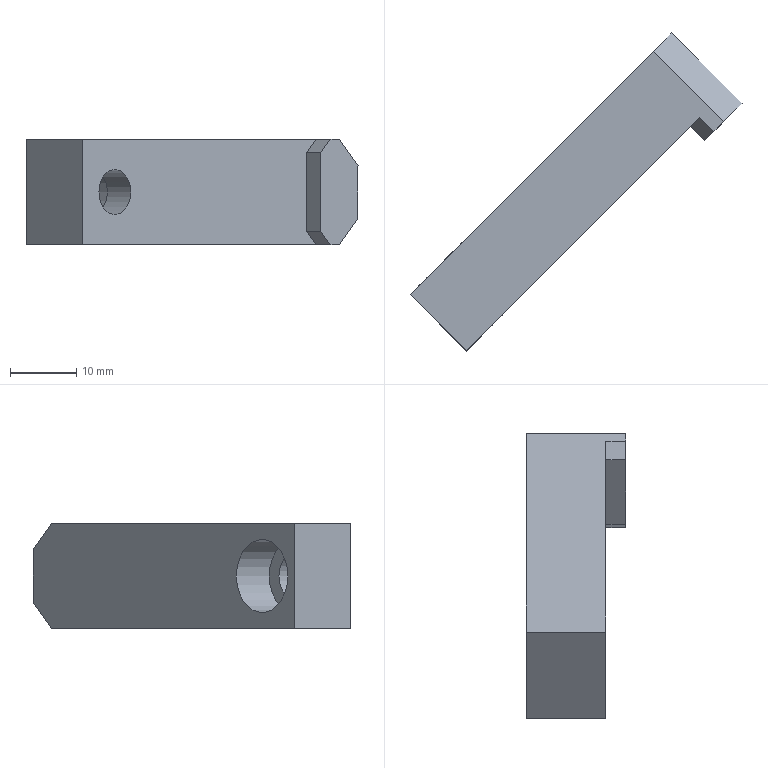Part | STEP file | gslz 2016.10.28-13_id1394_x_t | 1 solid | 15 faces | box 50.205 x 48.083 x 16 mm | volume 10037 mm3 | plane 13 | cylinder 2 | commonest cylinder face diameters 6.8 x1 11 x1
STEP:
#1=CARTESIAN_POINT('',(0.,0.,0.));
#2=DIRECTION('',(0.,0.,1.));
#3=DIRECTION('',(1.,0.,0.));
#4=AXIS2_PLACEMENT_3D('',#1,#2,#3);
#5=CARTESIAN_POINT('',(579.881,214.556,-16.623));
#6=VERTEX_POINT('',#5);
#7=CARTESIAN_POINT('',(578.467,213.142,-16.623));
#8=VERTEX_POINT('',#7);
#9=CARTESIAN_POINT('',(582.003,216.678,-16.623));
#10=DIRECTION('',(-0.7071,-0.7071,0.));
#11=VECTOR('',#10,1.);
#12=LINE('',#9,#11);
#13=CARTESIAN_POINT('',(562.204,215.264,-16.623));
#14=DIRECTION('',(0.,0.,-1.));
#15=DIRECTION('',(-0.766,0.6428,0.));
#16=AXIS2_PLACEMENT_3D('',#13,#14,#15);
#17=PLANE('',#16);
#18=CARTESIAN_POINT('',(-14.258,13.81));
#19=DIRECTION('',(0.08716,-0.9962));
#20=VECTOR('',#19,1.);
#21=LINE('',#18,#20);
#22=(GEOMETRIC_REPRESENTATION_CONTEXT(2)PARAMETRIC_REPRESENTATION_CONTEXT()REPRESENTATION_CONTEXT('',''));
#23=DEFINITIONAL_REPRESENTATION('',(#21),#22);
#24=PCURVE('',#17,#23);
#25=CARTESIAN_POINT('',(578.467,213.142,-46.123));
#26=DIRECTION('',(-0.7071,0.7071,0.));
#27=DIRECTION('',(-0.7071,-0.7071,0.));
#28=AXIS2_PLACEMENT_3D('',#25,#26,#27);
#29=PLANE('',#28);
#30=CARTESIAN_POINT('',(-5.,29.5));
#31=DIRECTION('',(1.,0.));
#32=VECTOR('',#31,1.);
#33=LINE('',#30,#32);
#34=(GEOMETRIC_REPRESENTATION_CONTEXT(2)PARAMETRIC_REPRESENTATION_CONTEXT()REPRESENTATION_CONTEXT('',''));
#35=DEFINITIONAL_REPRESENTATION('',(#33),#34);
#36=PCURVE('',#29,#35);
#37=SURFACE_CURVE('',#12,(#24,#36),.PCURVE_S1.);
#38=EDGE_CURVE('',#6,#8,#37,.T.);
#39=ORIENTED_EDGE('',*,*,#38,.F.);
#40=CARTESIAN_POINT('',(569.275,225.163,-16.623));
#41=VERTEX_POINT('',#40);
#42=CARTESIAN_POINT('',(569.275,225.163,-16.623));
#43=DIRECTION('',(-0.7071,0.7071,0.));
#44=VECTOR('',#43,1.);
#45=LINE('',#42,#44);
#46=CARTESIAN_POINT('',(0.9465,12.129));
#47=DIRECTION('',(0.9962,0.08716));
#48=VECTOR('',#47,1.);
#49=LINE('',#46,#48);
#50=(GEOMETRIC_REPRESENTATION_CONTEXT(2)PARAMETRIC_REPRESENTATION_CONTEXT()REPRESENTATION_CONTEXT('',''));
#51=DEFINITIONAL_REPRESENTATION('',(#49),#50);
#52=PCURVE('',#17,#51);
#53=CARTESIAN_POINT('',(570.689,223.749,-16.623));
#54=DIRECTION('',(0.5,0.5,0.7071));
#55=DIRECTION('',(0.7071,-0.7071,0.));
#56=AXIS2_PLACEMENT_3D('',#53,#54,#55);
#57=PLANE('',#56);
#58=CARTESIAN_POINT('',(-2.,0.));
#59=DIRECTION('',(-1.,0.));
#60=VECTOR('',#59,1.);
#61=LINE('',#58,#60);
#62=(GEOMETRIC_REPRESENTATION_CONTEXT(2)PARAMETRIC_REPRESENTATION_CONTEXT()REPRESENTATION_CONTEXT('',''));
#63=DEFINITIONAL_REPRESENTATION('',(#61),#62);
#64=PCURVE('',#57,#63);
#65=SURFACE_CURVE('',#45,(#52,#64),.PCURVE_S1.);
#66=EDGE_CURVE('',#6,#41,#65,.T.);
#67=ORIENTED_EDGE('',*,*,#66,.T.);
#68=CARTESIAN_POINT('',(532.505,188.393,-16.623));
#69=VERTEX_POINT('',#68);
#70=CARTESIAN_POINT('',(560.789,216.678,-16.623));
#71=DIRECTION('',(-0.7071,-0.7071,0.));
#72=VECTOR('',#71,1.);
#73=LINE('',#70,#72);
#74=CARTESIAN_POINT('',(1.992,0.1743));
#75=DIRECTION('',(0.08716,-0.9962));
#76=VECTOR('',#75,1.);
#77=LINE('',#74,#76);
#78=(GEOMETRIC_REPRESENTATION_CONTEXT(2)PARAMETRIC_REPRESENTATION_CONTEXT()REPRESENTATION_CONTEXT('',''));
#79=DEFINITIONAL_REPRESENTATION('',(#77),#78);
#80=PCURVE('',#17,#79);
#81=CARTESIAN_POINT('',(560.789,216.678,-46.123));
#82=DIRECTION('',(-0.7071,0.7071,0.));
#83=DIRECTION('',(-0.7071,-0.7071,0.));
#84=AXIS2_PLACEMENT_3D('',#81,#82,#83);
#85=PLANE('',#84);
#86=CARTESIAN_POINT('',(0.,29.5));
#87=DIRECTION('',(1.,0.));
#88=VECTOR('',#87,1.);
#89=LINE('',#86,#88);
#90=(GEOMETRIC_REPRESENTATION_CONTEXT(2)PARAMETRIC_REPRESENTATION_CONTEXT()REPRESENTATION_CONTEXT('',''));
#91=DEFINITIONAL_REPRESENTATION('',(#89),#90);
#92=PCURVE('',#85,#91);
#93=SURFACE_CURVE('',#73,(#80,#92),.PCURVE_S1.);
#94=EDGE_CURVE('',#41,#69,#93,.T.);
#95=ORIENTED_EDGE('',*,*,#94,.T.);
#96=CARTESIAN_POINT('',(540.99,179.908,-16.623));
#97=VERTEX_POINT('',#96);
#98=CARTESIAN_POINT('',(533.919,186.979,-16.623));
#99=DIRECTION('',(-0.7071,0.7071,0.));
#100=VECTOR('',#99,1.);
#101=LINE('',#98,#100);
#102=CARTESIAN_POINT('',(3.486,-39.848));
#103=DIRECTION('',(0.9962,0.08716));
#104=VECTOR('',#103,1.);
#105=LINE('',#102,#104);
#106=(GEOMETRIC_REPRESENTATION_CONTEXT(2)PARAMETRIC_REPRESENTATION_CONTEXT()REPRESENTATION_CONTEXT('',''));
#107=DEFINITIONAL_REPRESENTATION('',(#105),#106);
#108=PCURVE('',#17,#107);
#109=CARTESIAN_POINT('',(533.919,186.979,-46.123));
#110=DIRECTION('',(-0.7071,-0.7071,0.));
#111=DIRECTION('',(-0.7071,0.7071,0.));
#112=AXIS2_PLACEMENT_3D('',#109,#110,#111);
#113=PLANE('',#112);
#114=CARTESIAN_POINT('',(0.,-29.5));
#115=DIRECTION('',(1.,0.));
#116=VECTOR('',#115,1.);
#117=LINE('',#114,#116);
#118=(GEOMETRIC_REPRESENTATION_CONTEXT(2)PARAMETRIC_REPRESENTATION_CONTEXT()REPRESENTATION_CONTEXT('',''));
#119=DEFINITIONAL_REPRESENTATION('',(#117),#118);
#120=PCURVE('',#113,#119);
#121=SURFACE_CURVE('',#101,(#108,#120),.PCURVE_S1.);
#122=EDGE_CURVE('',#97,#69,#121,.T.);
#123=ORIENTED_EDGE('',*,*,#122,.F.);
#124=CARTESIAN_POINT('',(576.346,215.264,-16.623));
#125=VERTEX_POINT('',#124);
#126=CARTESIAN_POINT('',(569.275,208.192,-16.623));
#127=DIRECTION('',(-0.7071,-0.7071,0.));
#128=VECTOR('',#127,1.);
#129=LINE('',#126,#128);
#130=CARTESIAN_POINT('',(-9.962,-0.8716));
#131=DIRECTION('',(0.08716,-0.9962));
#132=VECTOR('',#131,1.);
#133=LINE('',#130,#132);
#134=(GEOMETRIC_REPRESENTATION_CONTEXT(2)PARAMETRIC_REPRESENTATION_CONTEXT()REPRESENTATION_CONTEXT('',''));
#135=DEFINITIONAL_REPRESENTATION('',(#133),#134);
#136=PCURVE('',#17,#135);
#137=CARTESIAN_POINT('',(569.275,208.192,-46.123));
#138=DIRECTION('',(-0.7071,0.7071,0.));
#139=DIRECTION('',(-0.7071,-0.7071,0.));
#140=AXIS2_PLACEMENT_3D('',#137,#138,#139);
#141=PLANE('',#140);
#142=CARTESIAN_POINT('',(0.,29.5));
#143=DIRECTION('',(1.,0.));
#144=VECTOR('',#143,1.);
#145=LINE('',#142,#144);
#146=(GEOMETRIC_REPRESENTATION_CONTEXT(2)PARAMETRIC_REPRESENTATION_CONTEXT()REPRESENTATION_CONTEXT('',''));
#147=DEFINITIONAL_REPRESENTATION('',(#145),#146);
#148=PCURVE('',#141,#147);
#149=SURFACE_CURVE('',#129,(#136,#148),.PCURVE_S1.);
#150=EDGE_CURVE('',#125,#97,#149,.T.);
#151=ORIENTED_EDGE('',*,*,#150,.F.);
#152=CARTESIAN_POINT('',(569.275,222.335,-16.623));
#153=DIRECTION('',(-0.7071,0.7071,0.));
#154=VECTOR('',#153,1.);
#155=LINE('',#152,#154);
#156=CARTESIAN_POINT('',(-0.8716,9.962));
#157=DIRECTION('',(0.9962,0.08716));
#158=VECTOR('',#157,1.);
#159=LINE('',#156,#158);
#160=(GEOMETRIC_REPRESENTATION_CONTEXT(2)PARAMETRIC_REPRESENTATION_CONTEXT()REPRESENTATION_CONTEXT('',''));
#161=DEFINITIONAL_REPRESENTATION('',(#159),#160);
#162=PCURVE('',#17,#161);
#163=CARTESIAN_POINT('',(570.689,223.749,-14.623));
#164=DIRECTION('',(0.5,0.5,-0.7071));
#165=DIRECTION('',(0.7071,-0.7071,0.));
#166=AXIS2_PLACEMENT_3D('',#163,#164,#165);
#167=PLANE('',#166);
#168=CARTESIAN_POINT('',(0.,2.828));
#169=DIRECTION('',(-1.,0.));
#170=VECTOR('',#169,1.);
#171=LINE('',#168,#170);
#172=(GEOMETRIC_REPRESENTATION_CONTEXT(2)PARAMETRIC_REPRESENTATION_CONTEXT()REPRESENTATION_CONTEXT('',''));
#173=DEFINITIONAL_REPRESENTATION('',(#171),#172);
#174=PCURVE('',#167,#173);
#175=SURFACE_CURVE('',#155,(#162,#174),.PCURVE_S1.);
#176=EDGE_CURVE('',#8,#125,#175,.T.);
#177=ORIENTED_EDGE('',*,*,#176,.F.);
#178=EDGE_LOOP('',(#39,#67,#95,#123,#151,#177));
#179=FACE_BOUND('',#178,.T.);
#180=ADVANCED_FACE('',(#179),#17,.F.);
#181=CARTESIAN_POINT('',(582.71,217.385,-20.623));
#182=VERTEX_POINT('',#181);
#183=CARTESIAN_POINT('',(582.71,217.385,-28.623));
#184=VERTEX_POINT('',#183);
#185=CARTESIAN_POINT('',(582.71,217.385,-46.123));
#186=DIRECTION('',(0.,0.,-1.));
#187=VECTOR('',#186,1.);
#188=LINE('',#185,#187);
#189=CARTESIAN_POINT('',(573.517,226.577,-46.123));
#190=DIRECTION('',(0.7071,0.7071,0.));
#191=DIRECTION('',(-0.7071,0.7071,0.));
#192=AXIS2_PLACEMENT_3D('',#189,#190,#191);
#193=PLANE('',#192);
#194=CARTESIAN_POINT('',(-13.,0.));
#195=DIRECTION('',(0.,-1.));
#196=VECTOR('',#195,1.);
#197=LINE('',#194,#196);
#198=(GEOMETRIC_REPRESENTATION_CONTEXT(2)PARAMETRIC_REPRESENTATION_CONTEXT()REPRESENTATION_CONTEXT('',''));
#199=DEFINITIONAL_REPRESENTATION('',(#197),#198);
#200=PCURVE('',#193,#199);
#201=CARTESIAN_POINT('',(-6.,0.));
#202=DIRECTION('',(0.,-1.));
#203=VECTOR('',#202,1.);
#204=LINE('',#201,#203);
#205=(GEOMETRIC_REPRESENTATION_CONTEXT(2)PARAMETRIC_REPRESENTATION_CONTEXT()REPRESENTATION_CONTEXT('',''));
#206=DEFINITIONAL_REPRESENTATION('',(#204),#205);
#207=PCURVE('',#29,#206);
#208=SURFACE_CURVE('',#188,(#200,#207),.PCURVE_S1.);
#209=EDGE_CURVE('',#182,#184,#208,.T.);
#210=ORIENTED_EDGE('',*,*,#209,.T.);
#211=CARTESIAN_POINT('',(572.103,227.991,-28.623));
#212=VERTEX_POINT('',#211);
#213=CARTESIAN_POINT('',(573.517,226.577,-28.623));
#214=DIRECTION('',(-0.7071,0.7071,0.));
#215=VECTOR('',#214,1.);
#216=LINE('',#213,#215);
#217=CARTESIAN_POINT('',(0.,17.5));
#218=DIRECTION('',(1.,0.));
#219=VECTOR('',#218,1.);
#220=LINE('',#217,#219);
#221=(GEOMETRIC_REPRESENTATION_CONTEXT(2)PARAMETRIC_REPRESENTATION_CONTEXT()REPRESENTATION_CONTEXT('',''));
#222=DEFINITIONAL_REPRESENTATION('',(#220),#221);
#223=PCURVE('',#193,#222);
#224=CARTESIAN_POINT('',(573.517,226.577,-28.623));
#225=DIRECTION('',(-0.5,-0.5,0.7071));
#226=DIRECTION('',(-0.7071,0.7071,0.));
#227=AXIS2_PLACEMENT_3D('',#224,#225,#226);
#228=PLANE('',#227);
#229=CARTESIAN_POINT('',(0.,0.));
#230=DIRECTION('',(1.,0.));
#231=VECTOR('',#230,1.);
#232=LINE('',#229,#231);
#233=(GEOMETRIC_REPRESENTATION_CONTEXT(2)PARAMETRIC_REPRESENTATION_CONTEXT()REPRESENTATION_CONTEXT('',''));
#234=DEFINITIONAL_REPRESENTATION('',(#232),#233);
#235=PCURVE('',#228,#234);
#236=SURFACE_CURVE('',#216,(#223,#235),.PCURVE_S1.);
#237=EDGE_CURVE('',#184,#212,#236,.T.);
#238=ORIENTED_EDGE('',*,*,#237,.T.);
#239=CARTESIAN_POINT('',(572.103,227.991,-20.623));
#240=VERTEX_POINT('',#239);
#241=CARTESIAN_POINT('',(572.103,227.991,-46.123));
#242=DIRECTION('',(0.,0.,1.));
#243=VECTOR('',#242,1.);
#244=LINE('',#241,#243);
#245=CARTESIAN_POINT('',(2.,0.));
#246=DIRECTION('',(0.,1.));
#247=VECTOR('',#246,1.);
#248=LINE('',#245,#247);
#249=(GEOMETRIC_REPRESENTATION_CONTEXT(2)PARAMETRIC_REPRESENTATION_CONTEXT()REPRESENTATION_CONTEXT('',''));
#250=DEFINITIONAL_REPRESENTATION('',(#248),#249);
#251=PCURVE('',#193,#250);
#252=CARTESIAN_POINT('',(-16.,0.));
#253=DIRECTION('',(0.,1.));
#254=VECTOR('',#253,1.);
#255=LINE('',#252,#254);
#256=(GEOMETRIC_REPRESENTATION_CONTEXT(2)PARAMETRIC_REPRESENTATION_CONTEXT()REPRESENTATION_CONTEXT('',''));
#257=DEFINITIONAL_REPRESENTATION('',(#255),#256);
#258=PCURVE('',#85,#257);
#259=SURFACE_CURVE('',#244,(#251,#258),.PCURVE_S1.);
#260=EDGE_CURVE('',#212,#240,#259,.T.);
#261=ORIENTED_EDGE('',*,*,#260,.T.);
#262=CARTESIAN_POINT('',(582.71,217.385,-20.623));
#263=DIRECTION('',(0.7071,-0.7071,0.));
#264=VECTOR('',#263,1.);
#265=LINE('',#262,#264);
#266=CARTESIAN_POINT('',(-13.,25.5));
#267=DIRECTION('',(-1.,0.));
#268=VECTOR('',#267,1.);
#269=LINE('',#266,#268);
#270=(GEOMETRIC_REPRESENTATION_CONTEXT(2)PARAMETRIC_REPRESENTATION_CONTEXT()REPRESENTATION_CONTEXT('',''));
#271=DEFINITIONAL_REPRESENTATION('',(#269),#270);
#272=PCURVE('',#193,#271);
#273=CARTESIAN_POINT('',(13.,5.657));
#274=DIRECTION('',(1.,0.));
#275=VECTOR('',#274,1.);
#276=LINE('',#273,#275);
#277=(GEOMETRIC_REPRESENTATION_CONTEXT(2)PARAMETRIC_REPRESENTATION_CONTEXT()REPRESENTATION_CONTEXT('',''));
#278=DEFINITIONAL_REPRESENTATION('',(#276),#277);
#279=PCURVE('',#57,#278);
#280=SURFACE_CURVE('',#265,(#272,#279),.PCURVE_S1.);
#281=EDGE_CURVE('',#240,#182,#280,.T.);
#282=ORIENTED_EDGE('',*,*,#281,.T.);
#283=EDGE_LOOP('',(#210,#238,#261,#282));
#284=FACE_BOUND('',#283,.T.);
#285=ADVANCED_FACE('',(#284),#193,.T.);
#286=ORIENTED_EDGE('',*,*,#260,.F.);
#287=CARTESIAN_POINT('',(569.275,225.163,-32.623));
#288=VERTEX_POINT('',#287);
#289=CARTESIAN_POINT('',(560.259,216.147,-45.373));
#290=DIRECTION('',(-0.5,-0.5,-0.7071));
#291=VECTOR('',#290,1.);
#292=LINE('',#289,#291);
#293=CARTESIAN_POINT('',(0.75,0.75));
#294=DIRECTION('',(0.7071,-0.7071));
#295=VECTOR('',#294,1.);
#296=LINE('',#293,#295);
#297=(GEOMETRIC_REPRESENTATION_CONTEXT(2)PARAMETRIC_REPRESENTATION_CONTEXT()REPRESENTATION_CONTEXT('',''));
#298=DEFINITIONAL_REPRESENTATION('',(#296),#297);
#299=PCURVE('',#85,#298);
#300=CARTESIAN_POINT('',(2.,23.688));
#301=DIRECTION('',(0.,1.));
#302=VECTOR('',#301,1.);
#303=LINE('',#300,#302);
#304=(GEOMETRIC_REPRESENTATION_CONTEXT(2)PARAMETRIC_REPRESENTATION_CONTEXT()REPRESENTATION_CONTEXT('',''));
#305=DEFINITIONAL_REPRESENTATION('',(#303),#304);
#306=PCURVE('',#228,#305);
#307=SURFACE_CURVE('',#292,(#299,#306),.PCURVE_S1.);
#308=EDGE_CURVE('',#212,#288,#307,.T.);
#309=ORIENTED_EDGE('',*,*,#308,.T.);
#310=CARTESIAN_POINT('',(532.505,188.393,-32.623));
#311=VERTEX_POINT('',#310);
#312=CARTESIAN_POINT('',(560.789,216.678,-32.623));
#313=DIRECTION('',(-0.7071,-0.7071,0.));
#314=VECTOR('',#313,1.);
#315=LINE('',#312,#314);
#316=CARTESIAN_POINT('',(0.,13.5));
#317=DIRECTION('',(1.,0.));
#318=VECTOR('',#317,1.);
#319=LINE('',#316,#318);
#320=(GEOMETRIC_REPRESENTATION_CONTEXT(2)PARAMETRIC_REPRESENTATION_CONTEXT()REPRESENTATION_CONTEXT('',''));
#321=DEFINITIONAL_REPRESENTATION('',(#319),#320);
#322=PCURVE('',#85,#321);
#323=CARTESIAN_POINT('',(562.204,215.264,-32.623));
#324=DIRECTION('',(0.,0.,-1.));
#325=DIRECTION('',(-0.766,0.6428,0.));
#326=AXIS2_PLACEMENT_3D('',#323,#324,#325);
#327=PLANE('',#326);
#328=CARTESIAN_POINT('',(1.992,0.1743));
#329=DIRECTION('',(0.08716,-0.9962));
#330=VECTOR('',#329,1.);
#331=LINE('',#328,#330);
#332=(GEOMETRIC_REPRESENTATION_CONTEXT(2)PARAMETRIC_REPRESENTATION_CONTEXT()REPRESENTATION_CONTEXT('',''));
#333=DEFINITIONAL_REPRESENTATION('',(#331),#332);
#334=PCURVE('',#327,#333);
#335=SURFACE_CURVE('',#315,(#322,#334),.PCURVE_S1.);
#336=EDGE_CURVE('',#288,#311,#335,.T.);
#337=ORIENTED_EDGE('',*,*,#336,.T.);
#338=CARTESIAN_POINT('',(532.505,188.393,-46.123));
#339=DIRECTION('',(0.,0.,-1.));
#340=VECTOR('',#339,1.);
#341=LINE('',#338,#340);
#342=CARTESIAN_POINT('',(40.,0.));
#343=DIRECTION('',(0.,-1.));
#344=VECTOR('',#343,1.);
#345=LINE('',#342,#344);
#346=(GEOMETRIC_REPRESENTATION_CONTEXT(2)PARAMETRIC_REPRESENTATION_CONTEXT()REPRESENTATION_CONTEXT('',''));
#347=DEFINITIONAL_REPRESENTATION('',(#345),#346);
#348=PCURVE('',#85,#347);
#349=CARTESIAN_POINT('',(2.,0.));
#350=DIRECTION('',(0.,1.));
#351=VECTOR('',#350,1.);
#352=LINE('',#349,#351);
#353=(GEOMETRIC_REPRESENTATION_CONTEXT(2)PARAMETRIC_REPRESENTATION_CONTEXT()REPRESENTATION_CONTEXT('',''));
#354=DEFINITIONAL_REPRESENTATION('',(#352),#353);
#355=PCURVE('',#113,#354);
#356=SURFACE_CURVE('',#341,(#348,#355),.PCURVE_S1.);
#357=EDGE_CURVE('',#69,#311,#356,.T.);
#358=ORIENTED_EDGE('',*,*,#357,.F.);
#359=ORIENTED_EDGE('',*,*,#94,.F.);
#360=CARTESIAN_POINT('',(575.462,231.35,-25.373));
#361=DIRECTION('',(0.5,0.5,-0.7071));
#362=VECTOR('',#361,1.);
#363=LINE('',#360,#362);
#364=CARTESIAN_POINT('',(-20.75,20.75));
#365=DIRECTION('',(-0.7071,-0.7071));
#366=VECTOR('',#365,1.);
#367=LINE('',#364,#366);
#368=(GEOMETRIC_REPRESENTATION_CONTEXT(2)PARAMETRIC_REPRESENTATION_CONTEXT()REPRESENTATION_CONTEXT('',''));
#369=DEFINITIONAL_REPRESENTATION('',(#367),#368);
#370=PCURVE('',#85,#369);
#371=CARTESIAN_POINT('',(-2.,12.374));
#372=DIRECTION('',(0.,1.));
#373=VECTOR('',#372,1.);
#374=LINE('',#371,#373);
#375=(GEOMETRIC_REPRESENTATION_CONTEXT(2)PARAMETRIC_REPRESENTATION_CONTEXT()REPRESENTATION_CONTEXT('',''));
#376=DEFINITIONAL_REPRESENTATION('',(#374),#375);
#377=PCURVE('',#57,#376);
#378=SURFACE_CURVE('',#363,(#370,#377),.PCURVE_S1.);
#379=EDGE_CURVE('',#41,#240,#378,.T.);
#380=ORIENTED_EDGE('',*,*,#379,.T.);
#381=EDGE_LOOP('',(#286,#309,#337,#358,#359,#380));
#382=FACE_BOUND('',#381,.T.);
#383=CARTESIAN_POINT('',(533.566,189.454,-24.623));
#384=VERTEX_POINT('',#383);
#385=CARTESIAN_POINT('',(541.344,197.232,-24.623));
#386=VERTEX_POINT('',#385);
#387=CARTESIAN_POINT('',(537.455,193.343,-24.623));
#388=DIRECTION('',(0.7071,-0.7071,0.));
#389=DIRECTION('',(-0.7071,-0.7071,0.));
#390=AXIS2_PLACEMENT_3D('',#387,#388,#389);
#391=CIRCLE('',#390,5.5);
#392=CARTESIAN_POINT('',(38.5,21.5));
#393=CARTESIAN_POINT('',(38.5,11.974));
#394=CARTESIAN_POINT('',(30.25,16.737));
#395=CARTESIAN_POINT('',(22.,21.5));
#396=CARTESIAN_POINT('',(30.25,26.263));
#397=CARTESIAN_POINT('',(38.5,31.026));
#398=CARTESIAN_POINT('',(38.5,21.5));
#399=(BOUNDED_CURVE()B_SPLINE_CURVE(2,(#392,#393,#394,#395,#396,#397,#398),.UNSPECIFIED.,.T.,.F.)B_SPLINE_CURVE_WITH_KNOTS((1,2,2,2,2,1),(-2.094,0.,2.094,4.189,6.283,8.378),.UNSPECIFIED.)CURVE()GEOMETRIC_REPRESENTATION_ITEM()RATIONAL_B_SPLINE_CURVE((1.,0.5,1.,0.5,1.,0.5,1.))REPRESENTATION_ITEM(''));
#400=(GEOMETRIC_REPRESENTATION_CONTEXT(2)PARAMETRIC_REPRESENTATION_CONTEXT()REPRESENTATION_CONTEXT('',''));
#401=DEFINITIONAL_REPRESENTATION('',(#399),#400);
#402=PCURVE('',#85,#401);
#403=CARTESIAN_POINT('',(533.212,197.586,-24.623));
#404=DIRECTION('',(0.7071,-0.7071,0.));
#405=DIRECTION('',(0.7071,0.7071,0.));
#406=AXIS2_PLACEMENT_3D('',#403,#404,#405);
#407=CYLINDRICAL_SURFACE('',#406,5.5);
#408=CARTESIAN_POINT('',(3.142,6.));
#409=DIRECTION('',(1.,0.));
#410=VECTOR('',#409,1.);
#411=LINE('',#408,#410);
#412=(GEOMETRIC_REPRESENTATION_CONTEXT(2)PARAMETRIC_REPRESENTATION_CONTEXT()REPRESENTATION_CONTEXT('',''));
#413=DEFINITIONAL_REPRESENTATION('',(#411),#412);
#414=PCURVE('',#407,#413);
#415=SURFACE_CURVE('',#391,(#402,#414),.PCURVE_S1.);
#416=EDGE_CURVE('',#384,#386,#415,.T.);
#417=ORIENTED_EDGE('',*,*,#416,.T.);
#418=CARTESIAN_POINT('',(537.455,193.343,-24.623));
#419=DIRECTION('',(0.7071,-0.7071,0.));
#420=DIRECTION('',(-0.7071,-0.7071,0.));
#421=AXIS2_PLACEMENT_3D('',#418,#419,#420);
#422=CIRCLE('',#421,5.5);
#423=CARTESIAN_POINT('',(38.5,21.5));
#424=CARTESIAN_POINT('',(38.5,11.974));
#425=CARTESIAN_POINT('',(30.25,16.737));
#426=CARTESIAN_POINT('',(22.,21.5));
#427=CARTESIAN_POINT('',(30.25,26.263));
#428=CARTESIAN_POINT('',(38.5,31.026));
#429=CARTESIAN_POINT('',(38.5,21.5));
#430=(BOUNDED_CURVE()B_SPLINE_CURVE(2,(#423,#424,#425,#426,#427,#428,#429),.UNSPECIFIED.,.T.,.F.)B_SPLINE_CURVE_WITH_KNOTS((1,2,2,2,2,1),(-2.094,0.,2.094,4.189,6.283,8.378),.UNSPECIFIED.)CURVE()GEOMETRIC_REPRESENTATION_ITEM()RATIONAL_B_SPLINE_CURVE((1.,0.5,1.,0.5,1.,0.5,1.))REPRESENTATION_ITEM(''));
#431=(GEOMETRIC_REPRESENTATION_CONTEXT(2)PARAMETRIC_REPRESENTATION_CONTEXT()REPRESENTATION_CONTEXT('',''));
#432=DEFINITIONAL_REPRESENTATION('',(#430),#431);
#433=PCURVE('',#85,#432);
#434=CARTESIAN_POINT('',(-3.142,6.));
#435=DIRECTION('',(1.,0.));
#436=VECTOR('',#435,1.);
#437=LINE('',#434,#436);
#438=(GEOMETRIC_REPRESENTATION_CONTEXT(2)PARAMETRIC_REPRESENTATION_CONTEXT()REPRESENTATION_CONTEXT('',''));
#439=DEFINITIONAL_REPRESENTATION('',(#437),#438);
#440=PCURVE('',#407,#439);
#441=SURFACE_CURVE('',#422,(#433,#440),.PCURVE_S1.);
#442=EDGE_CURVE('',#386,#384,#441,.T.);
#443=ORIENTED_EDGE('',*,*,#442,.T.);
#444=EDGE_LOOP('',(#417,#443));
#445=FACE_BOUND('',#444,.T.);
#446=ADVANCED_FACE('',(#382,#445),#85,.T.);
#447=CARTESIAN_POINT('',(576.346,215.264,-32.623));
#448=VERTEX_POINT('',#447);
#449=CARTESIAN_POINT('',(540.99,179.908,-32.623));
#450=VERTEX_POINT('',#449);
#451=CARTESIAN_POINT('',(569.275,208.192,-32.623));
#452=DIRECTION('',(-0.7071,-0.7071,0.));
#453=VECTOR('',#452,1.);
#454=LINE('',#451,#453);
#455=CARTESIAN_POINT('',(0.,13.5));
#456=DIRECTION('',(1.,0.));
#457=VECTOR('',#456,1.);
#458=LINE('',#455,#457);
#459=(GEOMETRIC_REPRESENTATION_CONTEXT(2)PARAMETRIC_REPRESENTATION_CONTEXT()REPRESENTATION_CONTEXT('',''));
#460=DEFINITIONAL_REPRESENTATION('',(#458),#459);
#461=PCURVE('',#141,#460);
#462=CARTESIAN_POINT('',(-9.962,-0.8716));
#463=DIRECTION('',(0.08716,-0.9962));
#464=VECTOR('',#463,1.);
#465=LINE('',#462,#464);
#466=(GEOMETRIC_REPRESENTATION_CONTEXT(2)PARAMETRIC_REPRESENTATION_CONTEXT()REPRESENTATION_CONTEXT('',''));
#467=DEFINITIONAL_REPRESENTATION('',(#465),#466);
#468=PCURVE('',#327,#467);
#469=SURFACE_CURVE('',#454,(#461,#468),.PCURVE_S1.);
#470=EDGE_CURVE('',#448,#450,#469,.T.);
#471=ORIENTED_EDGE('',*,*,#470,.F.);
#472=CARTESIAN_POINT('',(574.932,213.849,-30.623));
#473=VERTEX_POINT('',#472);
#474=CARTESIAN_POINT('',(574.048,212.965,-29.373));
#475=DIRECTION('',(0.5,0.5,-0.7071));
#476=VECTOR('',#475,1.);
#477=LINE('',#474,#476);
#478=CARTESIAN_POINT('',(-6.75,16.75));
#479=DIRECTION('',(-0.7071,-0.7071));
#480=VECTOR('',#479,1.);
#481=LINE('',#478,#480);
#482=(GEOMETRIC_REPRESENTATION_CONTEXT(2)PARAMETRIC_REPRESENTATION_CONTEXT()REPRESENTATION_CONTEXT('',''));
#483=DEFINITIONAL_REPRESENTATION('',(#481),#482);
#484=PCURVE('',#141,#483);
#485=CARTESIAN_POINT('',(570.689,223.749,-34.623));
#486=DIRECTION('',(-0.5,-0.5,-0.7071));
#487=DIRECTION('',(0.7071,-0.7071,0.));
#488=AXIS2_PLACEMENT_3D('',#485,#486,#487);
#489=PLANE('',#488);
#490=CARTESIAN_POINT('',(10.,7.425));
#491=DIRECTION('',(0.,-1.));
#492=VECTOR('',#491,1.);
#493=LINE('',#490,#492);
#494=(GEOMETRIC_REPRESENTATION_CONTEXT(2)PARAMETRIC_REPRESENTATION_CONTEXT()REPRESENTATION_CONTEXT('',''));
#495=DEFINITIONAL_REPRESENTATION('',(#493),#494);
#496=PCURVE('',#489,#495);
#497=SURFACE_CURVE('',#477,(#484,#496),.PCURVE_S1.);
#498=EDGE_CURVE('',#473,#448,#497,.T.);
#499=ORIENTED_EDGE('',*,*,#498,.F.);
#500=CARTESIAN_POINT('',(574.932,213.849,-18.623));
#501=VERTEX_POINT('',#500);
#502=CARTESIAN_POINT('',(574.932,213.849,-46.123));
#503=DIRECTION('',(0.,0.,1.));
#504=VECTOR('',#503,1.);
#505=LINE('',#502,#504);
#506=CARTESIAN_POINT('',(-8.,0.));
#507=DIRECTION('',(0.,1.));
#508=VECTOR('',#507,1.);
#509=LINE('',#506,#508);
#510=(GEOMETRIC_REPRESENTATION_CONTEXT(2)PARAMETRIC_REPRESENTATION_CONTEXT()REPRESENTATION_CONTEXT('',''));
#511=DEFINITIONAL_REPRESENTATION('',(#509),#510);
#512=PCURVE('',#141,#511);
#513=CARTESIAN_POINT('',(568.568,220.213,-24.623));
#514=DIRECTION('',(0.7071,0.7071,0.));
#515=DIRECTION('',(-0.7071,0.7071,0.));
#516=AXIS2_PLACEMENT_3D('',#513,#514,#515);
#517=PLANE('',#516);
#518=CARTESIAN_POINT('',(-9.,-21.5));
#519=DIRECTION('',(0.,1.));
#520=VECTOR('',#519,1.);
#521=LINE('',#518,#520);
#522=(GEOMETRIC_REPRESENTATION_CONTEXT(2)PARAMETRIC_REPRESENTATION_CONTEXT()REPRESENTATION_CONTEXT('',''));
#523=DEFINITIONAL_REPRESENTATION('',(#521),#522);
#524=PCURVE('',#517,#523);
#525=SURFACE_CURVE('',#505,(#512,#524),.PCURVE_S1.);
#526=EDGE_CURVE('',#473,#501,#525,.T.);
#527=ORIENTED_EDGE('',*,*,#526,.T.);
#528=CARTESIAN_POINT('',(558.845,197.763,-41.373));
#529=DIRECTION('',(-0.5,-0.5,-0.7071));
#530=VECTOR('',#529,1.);
#531=LINE('',#528,#530);
#532=CARTESIAN_POINT('',(14.75,4.75));
#533=DIRECTION('',(0.7071,-0.7071));
#534=VECTOR('',#533,1.);
#535=LINE('',#532,#534);
#536=(GEOMETRIC_REPRESENTATION_CONTEXT(2)PARAMETRIC_REPRESENTATION_CONTEXT()REPRESENTATION_CONTEXT('',''));
#537=DEFINITIONAL_REPRESENTATION('',(#535),#536);
#538=PCURVE('',#141,#537);
#539=CARTESIAN_POINT('',(10.,37.83));
#540=DIRECTION('',(0.,1.));
#541=VECTOR('',#540,1.);
#542=LINE('',#539,#541);
#543=(GEOMETRIC_REPRESENTATION_CONTEXT(2)PARAMETRIC_REPRESENTATION_CONTEXT()REPRESENTATION_CONTEXT('',''));
#544=DEFINITIONAL_REPRESENTATION('',(#542),#543);
#545=PCURVE('',#167,#544);
#546=SURFACE_CURVE('',#531,(#538,#545),.PCURVE_S1.);
#547=EDGE_CURVE('',#125,#501,#546,.T.);
#548=ORIENTED_EDGE('',*,*,#547,.F.);
#549=ORIENTED_EDGE('',*,*,#150,.T.);
#550=CARTESIAN_POINT('',(540.99,179.908,-46.123));
#551=DIRECTION('',(0.,0.,-1.));
#552=VECTOR('',#551,1.);
#553=LINE('',#550,#552);
#554=CARTESIAN_POINT('',(40.,0.));
#555=DIRECTION('',(0.,-1.));
#556=VECTOR('',#555,1.);
#557=LINE('',#554,#556);
#558=(GEOMETRIC_REPRESENTATION_CONTEXT(2)PARAMETRIC_REPRESENTATION_CONTEXT()REPRESENTATION_CONTEXT('',''));
#559=DEFINITIONAL_REPRESENTATION('',(#557),#558);
#560=PCURVE('',#141,#559);
#561=CARTESIAN_POINT('',(-10.,0.));
#562=DIRECTION('',(0.,1.));
#563=VECTOR('',#562,1.);
#564=LINE('',#561,#563);
#565=(GEOMETRIC_REPRESENTATION_CONTEXT(2)PARAMETRIC_REPRESENTATION_CONTEXT()REPRESENTATION_CONTEXT('',''));
#566=DEFINITIONAL_REPRESENTATION('',(#564),#565);
#567=PCURVE('',#113,#566);
#568=SURFACE_CURVE('',#553,(#560,#567),.PCURVE_S1.);
#569=EDGE_CURVE('',#97,#450,#568,.T.);
#570=ORIENTED_EDGE('',*,*,#569,.T.);
#571=EDGE_LOOP('',(#471,#499,#527,#548,#549,#570));
#572=FACE_BOUND('',#571,.T.);
#573=CARTESIAN_POINT('',(548.344,187.262,-24.623));
#574=VERTEX_POINT('',#573);
#575=CARTESIAN_POINT('',(545.94,184.858,-24.623));
#576=DIRECTION('',(-0.7071,0.7071,0.));
#577=DIRECTION('',(0.7071,0.7071,0.));
#578=AXIS2_PLACEMENT_3D('',#575,#576,#577);
#579=CIRCLE('',#578,3.4);
#580=CARTESIAN_POINT('',(33.,21.5));
#581=DIRECTION('',(-1.,0.));
#582=AXIS2_PLACEMENT_2D('',#580,#581);
#583=CIRCLE('',#582,3.4);
#584=(GEOMETRIC_REPRESENTATION_CONTEXT(2)PARAMETRIC_REPRESENTATION_CONTEXT()REPRESENTATION_CONTEXT('',''));
#585=DEFINITIONAL_REPRESENTATION('',(#583),#584);
#586=PCURVE('',#141,#585);
#587=CARTESIAN_POINT('',(611.701,119.097,-24.623));
#588=DIRECTION('',(0.7071,-0.7071,0.));
#589=DIRECTION('',(0.7071,0.7071,0.));
#590=AXIS2_PLACEMENT_3D('',#587,#588,#589);
#591=CYLINDRICAL_SURFACE('',#590,3.4);
#592=CARTESIAN_POINT('',(6.283,-93.));
#593=DIRECTION('',(-1.,0.));
#594=VECTOR('',#593,1.);
#595=LINE('',#592,#594);
#596=(GEOMETRIC_REPRESENTATION_CONTEXT(2)PARAMETRIC_REPRESENTATION_CONTEXT()REPRESENTATION_CONTEXT('',''));
#597=DEFINITIONAL_REPRESENTATION('',(#595),#596);
#598=PCURVE('',#591,#597);
#599=SURFACE_CURVE('',#579,(#586,#598),.PCURVE_S1.);
#600=EDGE_CURVE('',#574,#574,#599,.T.);
#601=ORIENTED_EDGE('',*,*,#600,.T.);
#602=EDGE_LOOP('',(#601));
#603=FACE_BOUND('',#602,.T.);
#604=ADVANCED_FACE('',(#572,#603),#141,.F.);
#605=ORIENTED_EDGE('',*,*,#336,.F.);
#606=CARTESIAN_POINT('',(579.881,214.556,-32.623));
#607=VERTEX_POINT('',#606);
#608=CARTESIAN_POINT('',(570.689,223.749,-32.623));
#609=DIRECTION('',(0.7071,-0.7071,0.));
#610=VECTOR('',#609,1.);
#611=LINE('',#608,#610);
#612=CARTESIAN_POINT('',(-1.046,11.954));
#613=DIRECTION('',(-0.9962,-0.08716));
#614=VECTOR('',#613,1.);
#615=LINE('',#612,#614);
#616=(GEOMETRIC_REPRESENTATION_CONTEXT(2)PARAMETRIC_REPRESENTATION_CONTEXT()REPRESENTATION_CONTEXT('',''));
#617=DEFINITIONAL_REPRESENTATION('',(#615),#616);
#618=PCURVE('',#327,#617);
#619=CARTESIAN_POINT('',(0.,5.657));
#620=DIRECTION('',(-1.,0.));
#621=VECTOR('',#620,1.);
#622=LINE('',#619,#621);
#623=(GEOMETRIC_REPRESENTATION_CONTEXT(2)PARAMETRIC_REPRESENTATION_CONTEXT()REPRESENTATION_CONTEXT('',''));
#624=DEFINITIONAL_REPRESENTATION('',(#622),#623);
#625=PCURVE('',#228,#624);
#626=SURFACE_CURVE('',#611,(#618,#625),.PCURVE_S1.);
#627=EDGE_CURVE('',#288,#607,#626,.T.);
#628=ORIENTED_EDGE('',*,*,#627,.T.);
#629=CARTESIAN_POINT('',(578.467,213.142,-32.623));
#630=VERTEX_POINT('',#629);
#631=CARTESIAN_POINT('',(582.003,216.678,-32.623));
#632=DIRECTION('',(-0.7071,-0.7071,0.));
#633=VECTOR('',#632,1.);
#634=LINE('',#631,#633);
#635=CARTESIAN_POINT('',(-14.258,13.81));
#636=DIRECTION('',(0.08716,-0.9962));
#637=VECTOR('',#636,1.);
#638=LINE('',#635,#637);
#639=(GEOMETRIC_REPRESENTATION_CONTEXT(2)PARAMETRIC_REPRESENTATION_CONTEXT()REPRESENTATION_CONTEXT('',''));
#640=DEFINITIONAL_REPRESENTATION('',(#638),#639);
#641=PCURVE('',#327,#640);
#642=CARTESIAN_POINT('',(-5.,13.5));
#643=DIRECTION('',(1.,0.));
#644=VECTOR('',#643,1.);
#645=LINE('',#642,#644);
#646=(GEOMETRIC_REPRESENTATION_CONTEXT(2)PARAMETRIC_REPRESENTATION_CONTEXT()REPRESENTATION_CONTEXT('',''));
#647=DEFINITIONAL_REPRESENTATION('',(#645),#646);
#648=PCURVE('',#29,#647);
#649=SURFACE_CURVE('',#634,(#641,#648),.PCURVE_S1.);
#650=EDGE_CURVE('',#607,#630,#649,.T.);
#651=ORIENTED_EDGE('',*,*,#650,.T.);
#652=CARTESIAN_POINT('',(569.275,222.335,-32.623));
#653=DIRECTION('',(0.7071,-0.7071,0.));
#654=VECTOR('',#653,1.);
#655=LINE('',#652,#654);
#656=CARTESIAN_POINT('',(-0.8716,9.962));
#657=DIRECTION('',(-0.9962,-0.08716));
#658=VECTOR('',#657,1.);
#659=LINE('',#656,#658);
#660=(GEOMETRIC_REPRESENTATION_CONTEXT(2)PARAMETRIC_REPRESENTATION_CONTEXT()REPRESENTATION_CONTEXT('',''));
#661=DEFINITIONAL_REPRESENTATION('',(#659),#660);
#662=PCURVE('',#327,#661);
#663=CARTESIAN_POINT('',(0.,2.828));
#664=DIRECTION('',(1.,0.));
#665=VECTOR('',#664,1.);
#666=LINE('',#663,#665);
#667=(GEOMETRIC_REPRESENTATION_CONTEXT(2)PARAMETRIC_REPRESENTATION_CONTEXT()REPRESENTATION_CONTEXT('',''));
#668=DEFINITIONAL_REPRESENTATION('',(#666),#667);
#669=PCURVE('',#489,#668);
#670=SURFACE_CURVE('',#655,(#662,#669),.PCURVE_S1.);
#671=EDGE_CURVE('',#448,#630,#670,.T.);
#672=ORIENTED_EDGE('',*,*,#671,.F.);
#673=ORIENTED_EDGE('',*,*,#470,.T.);
#674=CARTESIAN_POINT('',(533.919,186.979,-32.623));
#675=DIRECTION('',(-0.7071,0.7071,0.));
#676=VECTOR('',#675,1.);
#677=LINE('',#674,#676);
#678=CARTESIAN_POINT('',(3.486,-39.848));
#679=DIRECTION('',(0.9962,0.08716));
#680=VECTOR('',#679,1.);
#681=LINE('',#678,#680);
#682=(GEOMETRIC_REPRESENTATION_CONTEXT(2)PARAMETRIC_REPRESENTATION_CONTEXT()REPRESENTATION_CONTEXT('',''));
#683=DEFINITIONAL_REPRESENTATION('',(#681),#682);
#684=PCURVE('',#327,#683);
#685=CARTESIAN_POINT('',(0.,-13.5));
#686=DIRECTION('',(1.,0.));
#687=VECTOR('',#686,1.);
#688=LINE('',#685,#687);
#689=(GEOMETRIC_REPRESENTATION_CONTEXT(2)PARAMETRIC_REPRESENTATION_CONTEXT()REPRESENTATION_CONTEXT('',''));
#690=DEFINITIONAL_REPRESENTATION('',(#688),#689);
#691=PCURVE('',#113,#690);
#692=SURFACE_CURVE('',#677,(#684,#691),.PCURVE_S1.);
#693=EDGE_CURVE('',#450,#311,#692,.T.);
#694=ORIENTED_EDGE('',*,*,#693,.T.);
#695=EDGE_LOOP('',(#605,#628,#651,#672,#673,#694));
#696=FACE_BOUND('',#695,.T.);
#697=ADVANCED_FACE('',(#696),#327,.T.);
#698=ORIENTED_EDGE('',*,*,#650,.F.);
#699=CARTESIAN_POINT('',(582.71,217.385,-28.623));
#700=DIRECTION('',(0.5,0.5,0.7071));
#701=VECTOR('',#700,1.);
#702=LINE('',#699,#701);
#703=CARTESIAN_POINT('',(-6.,17.5));
#704=DIRECTION('',(-0.7071,0.7071));
#705=VECTOR('',#704,1.);
#706=LINE('',#703,#705);
#707=(GEOMETRIC_REPRESENTATION_CONTEXT(2)PARAMETRIC_REPRESENTATION_CONTEXT()REPRESENTATION_CONTEXT('',''));
#708=DEFINITIONAL_REPRESENTATION('',(#706),#707);
#709=PCURVE('',#29,#708);
#710=CARTESIAN_POINT('',(-13.,0.));
#711=DIRECTION('',(0.,-1.));
#712=VECTOR('',#711,1.);
#713=LINE('',#710,#712);
#714=(GEOMETRIC_REPRESENTATION_CONTEXT(2)PARAMETRIC_REPRESENTATION_CONTEXT()REPRESENTATION_CONTEXT('',''));
#715=DEFINITIONAL_REPRESENTATION('',(#713),#714);
#716=PCURVE('',#228,#715);
#717=SURFACE_CURVE('',#702,(#709,#716),.PCURVE_S1.);
#718=EDGE_CURVE('',#607,#184,#717,.T.);
#719=ORIENTED_EDGE('',*,*,#718,.T.);
#720=ORIENTED_EDGE('',*,*,#209,.F.);
#721=CARTESIAN_POINT('',(579.881,214.556,-16.623));
#722=DIRECTION('',(-0.5,-0.5,0.7071));
#723=VECTOR('',#722,1.);
#724=LINE('',#721,#723);
#725=CARTESIAN_POINT('',(-2.,29.5));
#726=DIRECTION('',(0.7071,0.7071));
#727=VECTOR('',#726,1.);
#728=LINE('',#725,#727);
#729=(GEOMETRIC_REPRESENTATION_CONTEXT(2)PARAMETRIC_REPRESENTATION_CONTEXT()REPRESENTATION_CONTEXT('',''));
#730=DEFINITIONAL_REPRESENTATION('',(#728),#729);
#731=PCURVE('',#29,#730);
#732=CARTESIAN_POINT('',(13.,0.));
#733=DIRECTION('',(0.,-1.));
#734=VECTOR('',#733,1.);
#735=LINE('',#732,#734);
#736=(GEOMETRIC_REPRESENTATION_CONTEXT(2)PARAMETRIC_REPRESENTATION_CONTEXT()REPRESENTATION_CONTEXT('',''));
#737=DEFINITIONAL_REPRESENTATION('',(#735),#736);
#738=PCURVE('',#57,#737);
#739=SURFACE_CURVE('',#724,(#731,#738),.PCURVE_S1.);
#740=EDGE_CURVE('',#182,#6,#739,.T.);
#741=ORIENTED_EDGE('',*,*,#740,.T.);
#742=ORIENTED_EDGE('',*,*,#38,.T.);
#743=CARTESIAN_POINT('',(577.053,211.728,-18.623));
#744=VERTEX_POINT('',#743);
#745=CARTESIAN_POINT('',(579.881,214.556,-14.623));
#746=DIRECTION('',(0.5,0.5,0.7071));
#747=VECTOR('',#746,1.);
#748=LINE('',#745,#747);
#749=CARTESIAN_POINT('',(-2.,31.5));
#750=DIRECTION('',(-0.7071,0.7071));
#751=VECTOR('',#750,1.);
#752=LINE('',#749,#751);
#753=(GEOMETRIC_REPRESENTATION_CONTEXT(2)PARAMETRIC_REPRESENTATION_CONTEXT()REPRESENTATION_CONTEXT('',''));
#754=DEFINITIONAL_REPRESENTATION('',(#752),#753);
#755=PCURVE('',#29,#754);
#756=CARTESIAN_POINT('',(13.,0.));
#757=DIRECTION('',(0.,-1.));
#758=VECTOR('',#757,1.);
#759=LINE('',#756,#758);
#760=(GEOMETRIC_REPRESENTATION_CONTEXT(2)PARAMETRIC_REPRESENTATION_CONTEXT()REPRESENTATION_CONTEXT('',''));
#761=DEFINITIONAL_REPRESENTATION('',(#759),#760);
#762=PCURVE('',#167,#761);
#763=SURFACE_CURVE('',#748,(#755,#762),.PCURVE_S1.);
#764=EDGE_CURVE('',#744,#8,#763,.T.);
#765=ORIENTED_EDGE('',*,*,#764,.F.);
#766=CARTESIAN_POINT('',(577.053,211.728,-30.623));
#767=VERTEX_POINT('',#766);
#768=CARTESIAN_POINT('',(577.053,211.728,-46.123));
#769=DIRECTION('',(0.,0.,-1.));
#770=VECTOR('',#769,1.);
#771=LINE('',#768,#770);
#772=CARTESIAN_POINT('',(2.,0.));
#773=DIRECTION('',(0.,-1.));
#774=VECTOR('',#773,1.);
#775=LINE('',#772,#774);
#776=(GEOMETRIC_REPRESENTATION_CONTEXT(2)PARAMETRIC_REPRESENTATION_CONTEXT()REPRESENTATION_CONTEXT('',''));
#777=DEFINITIONAL_REPRESENTATION('',(#775),#776);
#778=PCURVE('',#29,#777);
#779=CARTESIAN_POINT('',(-12.,-21.5));
#780=DIRECTION('',(0.,-1.));
#781=VECTOR('',#780,1.);
#782=LINE('',#779,#781);
#783=(GEOMETRIC_REPRESENTATION_CONTEXT(2)PARAMETRIC_REPRESENTATION_CONTEXT()REPRESENTATION_CONTEXT('',''));
#784=DEFINITIONAL_REPRESENTATION('',(#782),#783);
#785=PCURVE('',#517,#784);
#786=SURFACE_CURVE('',#771,(#778,#785),.PCURVE_S1.);
#787=EDGE_CURVE('',#744,#767,#786,.T.);
#788=ORIENTED_EDGE('',*,*,#787,.T.);
#789=CARTESIAN_POINT('',(579.881,214.556,-34.623));
#790=DIRECTION('',(-0.5,-0.5,0.7071));
#791=VECTOR('',#790,1.);
#792=LINE('',#789,#791);
#793=CARTESIAN_POINT('',(-2.,11.5));
#794=DIRECTION('',(0.7071,0.7071));
#795=VECTOR('',#794,1.);
#796=LINE('',#793,#795);
#797=(GEOMETRIC_REPRESENTATION_CONTEXT(2)PARAMETRIC_REPRESENTATION_CONTEXT()REPRESENTATION_CONTEXT('',''));
#798=DEFINITIONAL_REPRESENTATION('',(#796),#797);
#799=PCURVE('',#29,#798);
#800=CARTESIAN_POINT('',(13.,0.));
#801=DIRECTION('',(0.,1.));
#802=VECTOR('',#801,1.);
#803=LINE('',#800,#802);
#804=(GEOMETRIC_REPRESENTATION_CONTEXT(2)PARAMETRIC_REPRESENTATION_CONTEXT()REPRESENTATION_CONTEXT('',''));
#805=DEFINITIONAL_REPRESENTATION('',(#803),#804);
#806=PCURVE('',#489,#805);
#807=SURFACE_CURVE('',#792,(#799,#806),.PCURVE_S1.);
#808=EDGE_CURVE('',#630,#767,#807,.T.);
#809=ORIENTED_EDGE('',*,*,#808,.F.);
#810=EDGE_LOOP('',(#698,#719,#720,#741,#742,#765,#788,#809));
#811=FACE_BOUND('',#810,.T.);
#812=ADVANCED_FACE('',(#811),#29,.F.);
#813=ORIENTED_EDGE('',*,*,#787,.F.);
#814=CARTESIAN_POINT('',(568.568,220.213,-18.623));
#815=DIRECTION('',(0.7071,-0.7071,0.));
#816=VECTOR('',#815,1.);
#817=LINE('',#814,#816);
#818=CARTESIAN_POINT('',(0.,6.));
#819=DIRECTION('',(-1.,0.));
#820=VECTOR('',#819,1.);
#821=LINE('',#818,#820);
#822=(GEOMETRIC_REPRESENTATION_CONTEXT(2)PARAMETRIC_REPRESENTATION_CONTEXT()REPRESENTATION_CONTEXT('',''));
#823=DEFINITIONAL_REPRESENTATION('',(#821),#822);
#824=PCURVE('',#517,#823);
#825=CARTESIAN_POINT('',(1.,5.657));
#826=DIRECTION('',(1.,0.));
#827=VECTOR('',#826,1.);
#828=LINE('',#825,#827);
#829=(GEOMETRIC_REPRESENTATION_CONTEXT(2)PARAMETRIC_REPRESENTATION_CONTEXT()REPRESENTATION_CONTEXT('',''));
#830=DEFINITIONAL_REPRESENTATION('',(#828),#829);
#831=PCURVE('',#167,#830);
#832=SURFACE_CURVE('',#817,(#824,#831),.PCURVE_S1.);
#833=EDGE_CURVE('',#501,#744,#832,.T.);
#834=ORIENTED_EDGE('',*,*,#833,.F.);
#835=ORIENTED_EDGE('',*,*,#526,.F.);
#836=CARTESIAN_POINT('',(574.932,213.849,-30.623));
#837=DIRECTION('',(-0.7071,0.7071,0.));
#838=VECTOR('',#837,1.);
#839=LINE('',#836,#838);
#840=CARTESIAN_POINT('',(-9.,-6.));
#841=DIRECTION('',(1.,0.));
#842=VECTOR('',#841,1.);
#843=LINE('',#840,#842);
#844=(GEOMETRIC_REPRESENTATION_CONTEXT(2)PARAMETRIC_REPRESENTATION_CONTEXT()REPRESENTATION_CONTEXT('',''));
#845=DEFINITIONAL_REPRESENTATION('',(#843),#844);
#846=PCURVE('',#517,#845);
#847=CARTESIAN_POINT('',(10.,5.657));
#848=DIRECTION('',(-1.,0.));
#849=VECTOR('',#848,1.);
#850=LINE('',#847,#849);
#851=(GEOMETRIC_REPRESENTATION_CONTEXT(2)PARAMETRIC_REPRESENTATION_CONTEXT()REPRESENTATION_CONTEXT('',''));
#852=DEFINITIONAL_REPRESENTATION('',(#850),#851);
#853=PCURVE('',#489,#852);
#854=SURFACE_CURVE('',#839,(#846,#853),.PCURVE_S1.);
#855=EDGE_CURVE('',#767,#473,#854,.T.);
#856=ORIENTED_EDGE('',*,*,#855,.F.);
#857=EDGE_LOOP('',(#813,#834,#835,#856));
#858=FACE_BOUND('',#857,.T.);
#859=ADVANCED_FACE('',(#858),#517,.F.);
#860=ORIENTED_EDGE('',*,*,#357,.T.);
#861=ORIENTED_EDGE('',*,*,#693,.F.);
#862=ORIENTED_EDGE('',*,*,#569,.F.);
#863=ORIENTED_EDGE('',*,*,#122,.T.);
#864=EDGE_LOOP('',(#860,#861,#862,#863));
#865=FACE_BOUND('',#864,.T.);
#866=ADVANCED_FACE('',(#865),#113,.T.);
#867=CARTESIAN_POINT('',(544.809,190.798,-24.623));
#868=VERTEX_POINT('',#867);
#869=CARTESIAN_POINT('',(540.,185.989,-24.623));
#870=VERTEX_POINT('',#869);
#871=CARTESIAN_POINT('',(542.405,188.393,-24.623));
#872=DIRECTION('',(-0.7071,0.7071,0.));
#873=DIRECTION('',(-0.7071,-0.7071,0.));
#874=AXIS2_PLACEMENT_3D('',#871,#872,#873);
#875=CIRCLE('',#874,3.4);
#876=CARTESIAN_POINT('',(9.425,-98.));
#877=DIRECTION('',(-1.,0.));
#878=VECTOR('',#877,1.);
#879=LINE('',#876,#878);
#880=(GEOMETRIC_REPRESENTATION_CONTEXT(2)PARAMETRIC_REPRESENTATION_CONTEXT()REPRESENTATION_CONTEXT('',''));
#881=DEFINITIONAL_REPRESENTATION('',(#879),#880);
#882=PCURVE('',#591,#881);
#883=CARTESIAN_POINT('',(543.112,189.101,-24.623));
#884=DIRECTION('',(0.7071,-0.7071,0.));
#885=DIRECTION('',(0.7071,0.7071,0.));
#886=AXIS2_PLACEMENT_3D('',#883,#884,#885);
#887=PLANE('',#886);
#888=CARTESIAN_POINT('',(-4.4,-0.000000001));
#889=CARTESIAN_POINT('',(-4.4,5.889));
#890=CARTESIAN_POINT('',(0.7,2.944));
#891=CARTESIAN_POINT('',(5.8,0.000000001));
#892=CARTESIAN_POINT('',(0.7,-2.944));
#893=CARTESIAN_POINT('',(-4.4,-5.889));
#894=CARTESIAN_POINT('',(-4.4,-0.000000001));
#895=(BOUNDED_CURVE()B_SPLINE_CURVE(2,(#888,#889,#890,#891,#892,#893,#894),.UNSPECIFIED.,.T.,.F.)B_SPLINE_CURVE_WITH_KNOTS((1,2,2,2,2,1),(-2.094,0.,2.094,4.189,6.283,8.378),.UNSPECIFIED.)CURVE()GEOMETRIC_REPRESENTATION_ITEM()RATIONAL_B_SPLINE_CURVE((1.,0.5,1.,0.5,1.,0.5,1.))REPRESENTATION_ITEM(''));
#896=(GEOMETRIC_REPRESENTATION_CONTEXT(2)PARAMETRIC_REPRESENTATION_CONTEXT()REPRESENTATION_CONTEXT('',''));
#897=DEFINITIONAL_REPRESENTATION('',(#895),#896);
#898=PCURVE('',#887,#897);
#899=SURFACE_CURVE('',#875,(#882,#898),.PCURVE_S1.);
#900=EDGE_CURVE('',#868,#870,#899,.T.);
#901=ORIENTED_EDGE('',*,*,#900,.F.);
#902=CARTESIAN_POINT('',(544.809,190.798,-24.623));
#903=CARTESIAN_POINT('',(548.344,187.262,-24.623));
#904=B_SPLINE_CURVE_WITH_KNOTS('',1,(#902,#903),.UNSPECIFIED.,.F.,.F.,(2,2),(-98.,-93.),.PIECEWISE_BEZIER_KNOTS.);
#905=CARTESIAN_POINT('',(6.283,0.));
#906=DIRECTION('',(0.,1.));
#907=VECTOR('',#906,1.);
#908=LINE('',#905,#907);
#909=(GEOMETRIC_REPRESENTATION_CONTEXT(2)PARAMETRIC_REPRESENTATION_CONTEXT()REPRESENTATION_CONTEXT('',''));
#910=DEFINITIONAL_REPRESENTATION('',(#908),#909);
#911=PCURVE('',#591,#910);
#912=CARTESIAN_POINT('',(0.,0.));
#913=DIRECTION('',(0.,1.));
#914=VECTOR('',#913,1.);
#915=LINE('',#912,#914);
#916=(GEOMETRIC_REPRESENTATION_CONTEXT(2)PARAMETRIC_REPRESENTATION_CONTEXT()REPRESENTATION_CONTEXT('',''));
#917=DEFINITIONAL_REPRESENTATION('',(#915),#916);
#918=PCURVE('',#591,#917);
#919=SEAM_CURVE('',#904,(#911,#918),.PCURVE_S1.);
#920=EDGE_CURVE('',#868,#574,#919,.T.);
#921=ORIENTED_EDGE('',*,*,#920,.T.);
#922=ORIENTED_EDGE('',*,*,#600,.T.);
#923=ORIENTED_EDGE('',*,*,#920,.F.);
#924=CARTESIAN_POINT('',(542.405,188.393,-24.623));
#925=DIRECTION('',(-0.7071,0.7071,0.));
#926=DIRECTION('',(-0.7071,-0.7071,0.));
#927=AXIS2_PLACEMENT_3D('',#924,#925,#926);
#928=CIRCLE('',#927,3.4);
#929=CARTESIAN_POINT('',(3.142,-98.));
#930=DIRECTION('',(-1.,0.));
#931=VECTOR('',#930,1.);
#932=LINE('',#929,#931);
#933=(GEOMETRIC_REPRESENTATION_CONTEXT(2)PARAMETRIC_REPRESENTATION_CONTEXT()REPRESENTATION_CONTEXT('',''));
#934=DEFINITIONAL_REPRESENTATION('',(#932),#933);
#935=PCURVE('',#591,#934);
#936=CARTESIAN_POINT('',(-4.4,-0.000000001));
#937=CARTESIAN_POINT('',(-4.4,5.889));
#938=CARTESIAN_POINT('',(0.7,2.944));
#939=CARTESIAN_POINT('',(5.8,0.000000001));
#940=CARTESIAN_POINT('',(0.7,-2.944));
#941=CARTESIAN_POINT('',(-4.4,-5.889));
#942=CARTESIAN_POINT('',(-4.4,-0.000000001));
#943=(BOUNDED_CURVE()B_SPLINE_CURVE(2,(#936,#937,#938,#939,#940,#941,#942),.UNSPECIFIED.,.T.,.F.)B_SPLINE_CURVE_WITH_KNOTS((1,2,2,2,2,1),(-2.094,0.,2.094,4.189,6.283,8.378),.UNSPECIFIED.)CURVE()GEOMETRIC_REPRESENTATION_ITEM()RATIONAL_B_SPLINE_CURVE((1.,0.5,1.,0.5,1.,0.5,1.))REPRESENTATION_ITEM(''));
#944=(GEOMETRIC_REPRESENTATION_CONTEXT(2)PARAMETRIC_REPRESENTATION_CONTEXT()REPRESENTATION_CONTEXT('',''));
#945=DEFINITIONAL_REPRESENTATION('',(#943),#944);
#946=PCURVE('',#887,#945);
#947=SURFACE_CURVE('',#928,(#935,#946),.PCURVE_S1.);
#948=EDGE_CURVE('',#870,#868,#947,.T.);
#949=ORIENTED_EDGE('',*,*,#948,.F.);
#950=EDGE_LOOP('',(#901,#921,#922,#923,#949));
#951=FACE_BOUND('',#950,.F.);
#952=ADVANCED_FACE('',(#951),#591,.F.);
#953=ORIENTED_EDGE('',*,*,#948,.F.);
#954=ORIENTED_EDGE('',*,*,#900,.F.);
#955=EDGE_LOOP('',(#953,#954));
#956=FACE_BOUND('',#955,.T.);
#957=CARTESIAN_POINT('',(546.294,192.283,-24.623));
#958=VERTEX_POINT('',#957);
#959=CARTESIAN_POINT('',(542.405,188.393,-24.623));
#960=DIRECTION('',(-0.7071,0.7071,0.));
#961=DIRECTION('',(0.7071,0.7071,0.));
#962=AXIS2_PLACEMENT_3D('',#959,#960,#961);
#963=CIRCLE('',#962,5.5);
#964=CARTESIAN_POINT('',(4.5,0.000000001));
#965=CARTESIAN_POINT('',(4.5,-9.526));
#966=CARTESIAN_POINT('',(-3.75,-4.763));
#967=CARTESIAN_POINT('',(-12.,-0.000000002));
#968=CARTESIAN_POINT('',(-3.75,4.763));
#969=CARTESIAN_POINT('',(4.5,9.526));
#970=CARTESIAN_POINT('',(4.5,0.000000001));
#971=(BOUNDED_CURVE()B_SPLINE_CURVE(2,(#964,#965,#966,#967,#968,#969,#970),.UNSPECIFIED.,.T.,.F.)B_SPLINE_CURVE_WITH_KNOTS((1,2,2,2,2,1),(-2.094,0.,2.094,4.189,6.283,8.378),.UNSPECIFIED.)CURVE()GEOMETRIC_REPRESENTATION_ITEM()RATIONAL_B_SPLINE_CURVE((1.,0.5,1.,0.5,1.,0.5,1.))REPRESENTATION_ITEM(''));
#972=(GEOMETRIC_REPRESENTATION_CONTEXT(2)PARAMETRIC_REPRESENTATION_CONTEXT()REPRESENTATION_CONTEXT('',''));
#973=DEFINITIONAL_REPRESENTATION('',(#971),#972);
#974=PCURVE('',#887,#973);
#975=CARTESIAN_POINT('',(6.283,13.));
#976=DIRECTION('',(-1.,0.));
#977=VECTOR('',#976,1.);
#978=LINE('',#975,#977);
#979=(GEOMETRIC_REPRESENTATION_CONTEXT(2)PARAMETRIC_REPRESENTATION_CONTEXT()REPRESENTATION_CONTEXT('',''));
#980=DEFINITIONAL_REPRESENTATION('',(#978),#979);
#981=PCURVE('',#407,#980);
#982=SURFACE_CURVE('',#963,(#974,#981),.PCURVE_S1.);
#983=EDGE_CURVE('',#958,#958,#982,.T.);
#984=ORIENTED_EDGE('',*,*,#983,.T.);
#985=EDGE_LOOP('',(#984));
#986=FACE_BOUND('',#985,.T.);
#987=ADVANCED_FACE('',(#956,#986),#887,.F.);
#988=ORIENTED_EDGE('',*,*,#983,.T.);
#989=CARTESIAN_POINT('',(541.344,197.232,-24.623));
#990=CARTESIAN_POINT('',(546.294,192.283,-24.623));
#991=B_SPLINE_CURVE_WITH_KNOTS('',1,(#989,#990),.UNSPECIFIED.,.F.,.F.,(2,2),(6.,13.),.PIECEWISE_BEZIER_KNOTS.);
#992=CARTESIAN_POINT('',(0.,0.));
#993=DIRECTION('',(0.,1.));
#994=VECTOR('',#993,1.);
#995=LINE('',#992,#994);
#996=(GEOMETRIC_REPRESENTATION_CONTEXT(2)PARAMETRIC_REPRESENTATION_CONTEXT()REPRESENTATION_CONTEXT('',''));
#997=DEFINITIONAL_REPRESENTATION('',(#995),#996);
#998=PCURVE('',#407,#997);
#999=CARTESIAN_POINT('',(6.283,0.));
#1000=DIRECTION('',(0.,1.));
#1001=VECTOR('',#1000,1.);
#1002=LINE('',#999,#1001);
#1003=(GEOMETRIC_REPRESENTATION_CONTEXT(2)PARAMETRIC_REPRESENTATION_CONTEXT()REPRESENTATION_CONTEXT('',''));
#1004=DEFINITIONAL_REPRESENTATION('',(#1002),#1003);
#1005=PCURVE('',#407,#1004);
#1006=SEAM_CURVE('',#991,(#998,#1005),.PCURVE_S1.);
#1007=EDGE_CURVE('',#386,#958,#1006,.T.);
#1008=ORIENTED_EDGE('',*,*,#1007,.F.);
#1009=ORIENTED_EDGE('',*,*,#442,.T.);
#1010=ORIENTED_EDGE('',*,*,#416,.T.);
#1011=ORIENTED_EDGE('',*,*,#1007,.T.);
#1012=EDGE_LOOP('',(#988,#1008,#1009,#1010,#1011));
#1013=FACE_BOUND('',#1012,.F.);
#1014=ADVANCED_FACE('',(#1013),#407,.F.);
#1015=ORIENTED_EDGE('',*,*,#498,.T.);
#1016=ORIENTED_EDGE('',*,*,#671,.T.);
#1017=ORIENTED_EDGE('',*,*,#808,.T.);
#1018=ORIENTED_EDGE('',*,*,#855,.T.);
#1019=EDGE_LOOP('',(#1015,#1016,#1017,#1018));
#1020=FACE_BOUND('',#1019,.T.);
#1021=ADVANCED_FACE('',(#1020),#489,.T.);
#1022=ORIENTED_EDGE('',*,*,#764,.T.);
#1023=ORIENTED_EDGE('',*,*,#176,.T.);
#1024=ORIENTED_EDGE('',*,*,#547,.T.);
#1025=ORIENTED_EDGE('',*,*,#833,.T.);
#1026=EDGE_LOOP('',(#1022,#1023,#1024,#1025));
#1027=FACE_BOUND('',#1026,.T.);
#1028=ADVANCED_FACE('',(#1027),#167,.F.);
#1029=ORIENTED_EDGE('',*,*,#718,.F.);
#1030=ORIENTED_EDGE('',*,*,#627,.F.);
#1031=ORIENTED_EDGE('',*,*,#308,.F.);
#1032=ORIENTED_EDGE('',*,*,#237,.F.);
#1033=EDGE_LOOP('',(#1029,#1030,#1031,#1032));
#1034=FACE_BOUND('',#1033,.T.);
#1035=ADVANCED_FACE('',(#1034),#228,.F.);
#1036=ORIENTED_EDGE('',*,*,#740,.F.);
#1037=ORIENTED_EDGE('',*,*,#281,.F.);
#1038=ORIENTED_EDGE('',*,*,#379,.F.);
#1039=ORIENTED_EDGE('',*,*,#66,.F.);
#1040=EDGE_LOOP('',(#1036,#1037,#1038,#1039));
#1041=FACE_BOUND('',#1040,.T.);
#1042=ADVANCED_FACE('',(#1041),#57,.T.);
#1043=CLOSED_SHELL('',(#180,#285,#446,#604,#697,#812,#859,#866,#952,#987,#1014,#1021,#1028,#1035,#1042));
#1044=MANIFOLD_SOLID_BREP('',#1043);
#1045=(LENGTH_UNIT()NAMED_UNIT(*)SI_UNIT(.MILLI.,.METRE.));
#1046=UNCERTAINTY_MEASURE_WITH_UNIT(LENGTH_MEASURE(0.000001),#1045,'','');
#1047=(NAMED_UNIT(*)PLANE_ANGLE_UNIT()SI_UNIT($,.RADIAN.));
#1048=(NAMED_UNIT(*)SI_UNIT($,.STERADIAN.)SOLID_ANGLE_UNIT());
#1049=(GEOMETRIC_REPRESENTATION_CONTEXT(3)GLOBAL_UNCERTAINTY_ASSIGNED_CONTEXT((#1046))GLOBAL_UNIT_ASSIGNED_CONTEXT((#1045,#1047,#1048))REPRESENTATION_CONTEXT('',''));
#1050=ADVANCED_BREP_SHAPE_REPRESENTATION('',(#4,#1044),#1049);